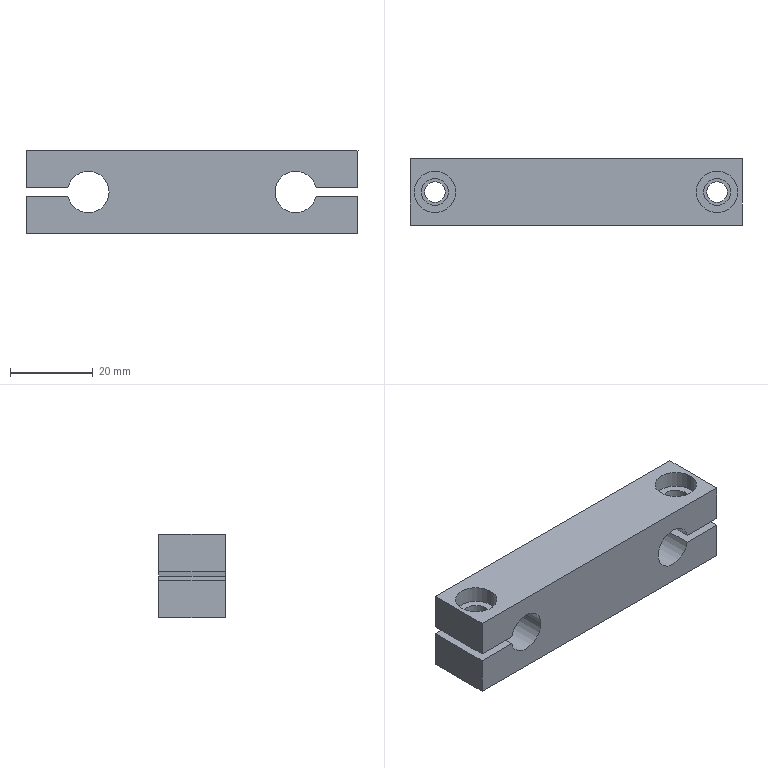Part | SolidWorks | features ICE 4, Extrusion 1, HoleWzd 1 | 1 solid | 29 faces | box 80 x 16 x 20 mm | volume 21131 mm3 | cylinder 15 | plane 14 | commonest cylinder face diameters 10 x7 5 x4 6.5 x4
STEP:
#1=CARTESIAN_POINT('',(-79.,8.,16.));
#2=VERTEX_POINT('',#1);
#3=CARTESIAN_POINT('',(-69.,8.,16.));
#4=VERTEX_POINT('',#3);
#5=CARTESIAN_POINT('',(-74.,8.,16.));
#6=DIRECTION('',(0.,0.,1.));
#7=DIRECTION('',(1.,0.,0.));
#8=AXIS2_PLACEMENT_3D('',#5,#6,#7);
#9=CIRCLE('',#8,5.);
#10=EDGE_CURVE('',#2,#4,#9,.T.);
#11=ORIENTED_EDGE('',*,*,#10,.F.);
#12=CARTESIAN_POINT('',(-79.,8.,20.));
#13=VERTEX_POINT('',#12);
#14=CARTESIAN_POINT('',(-79.,8.,16.));
#15=DIRECTION('',(0.,0.,1.));
#16=VECTOR('',#15,1000.);
#17=LINE('',#14,#16);
#18=EDGE_CURVE('',#2,#13,#17,.T.);
#19=ORIENTED_EDGE('',*,*,#18,.T.);
#20=CARTESIAN_POINT('',(-69.,8.,20.));
#21=VERTEX_POINT('',#20);
#22=CARTESIAN_POINT('',(-74.,8.,20.));
#23=DIRECTION('',(0.,0.,1.));
#24=DIRECTION('',(1.,0.,0.));
#25=AXIS2_PLACEMENT_3D('',#22,#23,#24);
#26=CIRCLE('',#25,5.);
#27=EDGE_CURVE('',#13,#21,#26,.T.);
#28=ORIENTED_EDGE('',*,*,#27,.T.);
#29=CARTESIAN_POINT('',(-69.,8.,16.));
#30=DIRECTION('',(0.,0.,1.));
#31=VECTOR('',#30,1000.);
#32=LINE('',#29,#31);
#33=EDGE_CURVE('',#4,#21,#32,.T.);
#34=ORIENTED_EDGE('',*,*,#33,.F.);
#35=EDGE_LOOP('',(#11,#19,#28,#34));
#36=FACE_OUTER_BOUND('',#35,.T.);
#37=CARTESIAN_POINT('',(-74.,8.,16.));
#38=DIRECTION('',(0.,0.,1.));
#39=DIRECTION('',(1.,0.,0.));
#40=AXIS2_PLACEMENT_3D('',#37,#38,#39);
#41=CYLINDRICAL_SURFACE('',#40,5.);
#42=ADVANCED_FACE('',(#36),#41,.F.);
#43=CARTESIAN_POINT('',(-11.,8.,16.));
#44=VERTEX_POINT('',#43);
#45=CARTESIAN_POINT('',(-1.,8.,16.));
#46=VERTEX_POINT('',#45);
#47=CARTESIAN_POINT('',(-6.,8.,16.));
#48=DIRECTION('',(0.,0.,1.));
#49=DIRECTION('',(1.,0.,0.));
#50=AXIS2_PLACEMENT_3D('',#47,#48,#49);
#51=CIRCLE('',#50,5.);
#52=EDGE_CURVE('',#44,#46,#51,.T.);
#53=ORIENTED_EDGE('',*,*,#52,.F.);
#54=CARTESIAN_POINT('',(-11.,8.,20.));
#55=VERTEX_POINT('',#54);
#56=CARTESIAN_POINT('',(-11.,8.,16.));
#57=DIRECTION('',(0.,0.,1.));
#58=VECTOR('',#57,1000.);
#59=LINE('',#56,#58);
#60=EDGE_CURVE('',#44,#55,#59,.T.);
#61=ORIENTED_EDGE('',*,*,#60,.T.);
#62=CARTESIAN_POINT('',(-1.,8.,20.));
#63=VERTEX_POINT('',#62);
#64=CARTESIAN_POINT('',(-6.,8.,20.));
#65=DIRECTION('',(0.,0.,1.));
#66=DIRECTION('',(1.,0.,0.));
#67=AXIS2_PLACEMENT_3D('',#64,#65,#66);
#68=CIRCLE('',#67,5.);
#69=EDGE_CURVE('',#55,#63,#68,.T.);
#70=ORIENTED_EDGE('',*,*,#69,.T.);
#71=CARTESIAN_POINT('',(-1.,8.,16.));
#72=DIRECTION('',(0.,0.,1.));
#73=VECTOR('',#72,1000.);
#74=LINE('',#71,#73);
#75=EDGE_CURVE('',#46,#63,#74,.T.);
#76=ORIENTED_EDGE('',*,*,#75,.F.);
#77=EDGE_LOOP('',(#53,#61,#70,#76));
#78=FACE_OUTER_BOUND('',#77,.T.);
#79=CARTESIAN_POINT('',(-6.,8.,16.));
#80=DIRECTION('',(0.,0.,1.));
#81=DIRECTION('',(1.,0.,0.));
#82=AXIS2_PLACEMENT_3D('',#79,#80,#81);
#83=CYLINDRICAL_SURFACE('',#82,5.);
#84=ADVANCED_FACE('',(#78),#83,.F.);
#85=CARTESIAN_POINT('',(-8.5,8.,0.));
#86=VERTEX_POINT('',#85);
#87=CARTESIAN_POINT('',(-3.5,8.,0.));
#88=VERTEX_POINT('',#87);
#89=CARTESIAN_POINT('',(-6.,8.,0.));
#90=DIRECTION('',(0.,0.,1.));
#91=DIRECTION('',(1.,0.,0.));
#92=AXIS2_PLACEMENT_3D('',#89,#90,#91);
#93=CIRCLE('',#92,2.5);
#94=EDGE_CURVE('',#86,#88,#93,.T.);
#95=ORIENTED_EDGE('',*,*,#94,.F.);
#96=CARTESIAN_POINT('',(-8.5,8.,9.));
#97=VERTEX_POINT('',#96);
#98=CARTESIAN_POINT('',(-8.5,8.,9.));
#99=DIRECTION('',(0.,0.,1.));
#100=VECTOR('',#99,1000.);
#101=LINE('',#98,#100);
#102=EDGE_CURVE('',#86,#97,#101,.T.);
#103=ORIENTED_EDGE('',*,*,#102,.T.);
#104=CARTESIAN_POINT('',(-3.5,8.,9.));
#105=VERTEX_POINT('',#104);
#106=CARTESIAN_POINT('',(-6.,8.,9.));
#107=DIRECTION('',(0.,0.,1.));
#108=DIRECTION('',(1.,0.,0.));
#109=AXIS2_PLACEMENT_3D('',#106,#107,#108);
#110=CIRCLE('',#109,2.5);
#111=EDGE_CURVE('',#97,#105,#110,.T.);
#112=ORIENTED_EDGE('',*,*,#111,.T.);
#113=CARTESIAN_POINT('',(-3.5,8.,9.));
#114=DIRECTION('',(0.,0.,1.));
#115=VECTOR('',#114,1000.);
#116=LINE('',#113,#115);
#117=EDGE_CURVE('',#88,#105,#116,.T.);
#118=ORIENTED_EDGE('',*,*,#117,.F.);
#119=EDGE_LOOP('',(#95,#103,#112,#118));
#120=FACE_OUTER_BOUND('',#119,.T.);
#121=CARTESIAN_POINT('',(-6.,8.,9.));
#122=DIRECTION('',(0.,0.,1.));
#123=DIRECTION('',(1.,0.,0.));
#124=AXIS2_PLACEMENT_3D('',#121,#122,#123);
#125=CYLINDRICAL_SURFACE('',#124,2.5);
#126=ADVANCED_FACE('',(#120),#125,.F.);
#127=CARTESIAN_POINT('',(-76.5,8.,0.));
#128=VERTEX_POINT('',#127);
#129=CARTESIAN_POINT('',(-71.5,8.,0.));
#130=VERTEX_POINT('',#129);
#131=CARTESIAN_POINT('',(-74.,8.,0.));
#132=DIRECTION('',(0.,0.,1.));
#133=DIRECTION('',(1.,0.,0.));
#134=AXIS2_PLACEMENT_3D('',#131,#132,#133);
#135=CIRCLE('',#134,2.5);
#136=EDGE_CURVE('',#128,#130,#135,.T.);
#137=ORIENTED_EDGE('',*,*,#136,.F.);
#138=CARTESIAN_POINT('',(-76.5,8.,9.));
#139=VERTEX_POINT('',#138);
#140=CARTESIAN_POINT('',(-76.5,8.,9.));
#141=DIRECTION('',(0.,0.,1.));
#142=VECTOR('',#141,1000.);
#143=LINE('',#140,#142);
#144=EDGE_CURVE('',#128,#139,#143,.T.);
#145=ORIENTED_EDGE('',*,*,#144,.T.);
#146=CARTESIAN_POINT('',(-71.5,8.,9.));
#147=VERTEX_POINT('',#146);
#148=CARTESIAN_POINT('',(-74.,8.,9.));
#149=DIRECTION('',(0.,0.,1.));
#150=DIRECTION('',(1.,0.,0.));
#151=AXIS2_PLACEMENT_3D('',#148,#149,#150);
#152=CIRCLE('',#151,2.5);
#153=EDGE_CURVE('',#139,#147,#152,.T.);
#154=ORIENTED_EDGE('',*,*,#153,.T.);
#155=CARTESIAN_POINT('',(-71.5,8.,9.));
#156=DIRECTION('',(0.,0.,1.));
#157=VECTOR('',#156,1000.);
#158=LINE('',#155,#157);
#159=EDGE_CURVE('',#130,#147,#158,.T.);
#160=ORIENTED_EDGE('',*,*,#159,.F.);
#161=EDGE_LOOP('',(#137,#145,#154,#160));
#162=FACE_OUTER_BOUND('',#161,.T.);
#163=CARTESIAN_POINT('',(-74.,8.,9.));
#164=DIRECTION('',(0.,0.,1.));
#165=DIRECTION('',(1.,0.,0.));
#166=AXIS2_PLACEMENT_3D('',#163,#164,#165);
#167=CYLINDRICAL_SURFACE('',#166,2.5);
#168=ADVANCED_FACE('',(#162),#167,.F.);
#169=CARTESIAN_POINT('',(-60.,16.,10.));
#170=VERTEX_POINT('',#169);
#171=CARTESIAN_POINT('',(-69.899,16.,11.));
#172=VERTEX_POINT('',#171);
#173=CARTESIAN_POINT('',(-65.,16.,10.));
#174=DIRECTION('',(0.,-1.,0.));
#175=DIRECTION('',(1.,0.,0.));
#176=AXIS2_PLACEMENT_3D('',#173,#174,#175);
#177=CIRCLE('',#176,5.);
#178=EDGE_CURVE('',#170,#172,#177,.T.);
#179=ORIENTED_EDGE('',*,*,#178,.F.);
#180=CARTESIAN_POINT('',(-60.,0.,10.));
#181=VERTEX_POINT('',#180);
#182=CARTESIAN_POINT('',(-60.,20.,10.));
#183=DIRECTION('',(0.,-1.,0.));
#184=VECTOR('',#183,1000.);
#185=LINE('',#182,#184);
#186=EDGE_CURVE('',#170,#181,#185,.T.);
#187=ORIENTED_EDGE('',*,*,#186,.T.);
#188=CARTESIAN_POINT('',(-69.899,0.,11.));
#189=VERTEX_POINT('',#188);
#190=CARTESIAN_POINT('',(-65.,0.,10.));
#191=DIRECTION('',(0.,-1.,0.));
#192=DIRECTION('',(1.,0.,0.));
#193=AXIS2_PLACEMENT_3D('',#190,#191,#192);
#194=CIRCLE('',#193,5.);
#195=EDGE_CURVE('',#181,#189,#194,.T.);
#196=ORIENTED_EDGE('',*,*,#195,.T.);
#197=CARTESIAN_POINT('',(-69.899,20.,11.));
#198=DIRECTION('',(0.,1.,0.));
#199=VECTOR('',#198,1000.);
#200=LINE('',#197,#199);
#201=EDGE_CURVE('',#189,#172,#200,.T.);
#202=ORIENTED_EDGE('',*,*,#201,.T.);
#203=EDGE_LOOP('',(#179,#187,#196,#202));
#204=FACE_OUTER_BOUND('',#203,.T.);
#205=CARTESIAN_POINT('',(-65.,20.,10.));
#206=DIRECTION('',(0.,-1.,0.));
#207=DIRECTION('',(1.,0.,0.));
#208=AXIS2_PLACEMENT_3D('',#205,#206,#207);
#209=CYLINDRICAL_SURFACE('',#208,5.);
#210=ADVANCED_FACE('',(#204),#209,.F.);
#211=CARTESIAN_POINT('',(-2.75,8.,16.));
#212=VERTEX_POINT('',#211);
#213=CARTESIAN_POINT('',(-9.25,8.,16.));
#214=VERTEX_POINT('',#213);
#215=CARTESIAN_POINT('',(-6.,8.,16.));
#216=DIRECTION('',(0.,0.,-1.));
#217=DIRECTION('',(1.,0.,0.));
#218=AXIS2_PLACEMENT_3D('',#215,#216,#217);
#219=CIRCLE('',#218,3.25);
#220=EDGE_CURVE('',#212,#214,#219,.T.);
#221=ORIENTED_EDGE('',*,*,#220,.F.);
#222=CARTESIAN_POINT('',(-2.75,8.,11.));
#223=VERTEX_POINT('',#222);
#224=CARTESIAN_POINT('',(-2.75,8.,41.));
#225=DIRECTION('',(0.,0.,-1.));
#226=VECTOR('',#225,1000.);
#227=LINE('',#224,#226);
#228=EDGE_CURVE('',#212,#223,#227,.T.);
#229=ORIENTED_EDGE('',*,*,#228,.T.);
#230=CARTESIAN_POINT('',(-9.25,8.,11.));
#231=VERTEX_POINT('',#230);
#232=CARTESIAN_POINT('',(-6.,8.,11.));
#233=DIRECTION('',(0.,0.,-1.));
#234=DIRECTION('',(-1.,0.,0.));
#235=AXIS2_PLACEMENT_3D('',#232,#233,#234);
#236=CIRCLE('',#235,3.25);
#237=EDGE_CURVE('',#223,#231,#236,.T.);
#238=ORIENTED_EDGE('',*,*,#237,.T.);
#239=CARTESIAN_POINT('',(-9.25,8.,41.));
#240=DIRECTION('',(0.,0.,-1.));
#241=VECTOR('',#240,1000.);
#242=LINE('',#239,#241);
#243=EDGE_CURVE('',#214,#231,#242,.T.);
#244=ORIENTED_EDGE('',*,*,#243,.F.);
#245=EDGE_LOOP('',(#221,#229,#238,#244));
#246=FACE_OUTER_BOUND('',#245,.T.);
#247=CARTESIAN_POINT('',(-6.,8.,41.));
#248=DIRECTION('',(0.,0.,-1.));
#249=DIRECTION('',(-1.,0.,0.));
#250=AXIS2_PLACEMENT_3D('',#247,#248,#249);
#251=CYLINDRICAL_SURFACE('',#250,3.25);
#252=ADVANCED_FACE('',(#246),#251,.F.);
#253=CARTESIAN_POINT('',(-70.75,8.,16.));
#254=VERTEX_POINT('',#253);
#255=CARTESIAN_POINT('',(-77.25,8.,16.));
#256=VERTEX_POINT('',#255);
#257=CARTESIAN_POINT('',(-74.,8.,16.));
#258=DIRECTION('',(0.,0.,-1.));
#259=DIRECTION('',(1.,0.,0.));
#260=AXIS2_PLACEMENT_3D('',#257,#258,#259);
#261=CIRCLE('',#260,3.25);
#262=EDGE_CURVE('',#254,#256,#261,.T.);
#263=ORIENTED_EDGE('',*,*,#262,.F.);
#264=CARTESIAN_POINT('',(-70.75,8.,11.));
#265=VERTEX_POINT('',#264);
#266=CARTESIAN_POINT('',(-70.75,8.,41.));
#267=DIRECTION('',(0.,0.,-1.));
#268=VECTOR('',#267,1000.);
#269=LINE('',#266,#268);
#270=EDGE_CURVE('',#254,#265,#269,.T.);
#271=ORIENTED_EDGE('',*,*,#270,.T.);
#272=CARTESIAN_POINT('',(-77.25,8.,11.));
#273=VERTEX_POINT('',#272);
#274=CARTESIAN_POINT('',(-74.,8.,11.));
#275=DIRECTION('',(0.,0.,-1.));
#276=DIRECTION('',(-1.,0.,0.));
#277=AXIS2_PLACEMENT_3D('',#274,#275,#276);
#278=CIRCLE('',#277,3.25);
#279=EDGE_CURVE('',#265,#273,#278,.T.);
#280=ORIENTED_EDGE('',*,*,#279,.T.);
#281=CARTESIAN_POINT('',(-77.25,8.,41.));
#282=DIRECTION('',(0.,0.,-1.));
#283=VECTOR('',#282,1000.);
#284=LINE('',#281,#283);
#285=EDGE_CURVE('',#256,#273,#284,.T.);
#286=ORIENTED_EDGE('',*,*,#285,.F.);
#287=EDGE_LOOP('',(#263,#271,#280,#286));
#288=FACE_OUTER_BOUND('',#287,.T.);
#289=CARTESIAN_POINT('',(-74.,8.,41.));
#290=DIRECTION('',(0.,0.,-1.));
#291=DIRECTION('',(-1.,0.,0.));
#292=AXIS2_PLACEMENT_3D('',#289,#290,#291);
#293=CYLINDRICAL_SURFACE('',#292,3.25);
#294=ADVANCED_FACE('',(#288),#293,.F.);
#295=ORIENTED_EDGE('',*,*,#270,.F.);
#296=CARTESIAN_POINT('',(-74.,8.,16.));
#297=DIRECTION('',(0.,0.,-1.));
#298=DIRECTION('',(1.,0.,0.));
#299=AXIS2_PLACEMENT_3D('',#296,#297,#298);
#300=CIRCLE('',#299,3.25);
#301=EDGE_CURVE('',#256,#254,#300,.T.);
#302=ORIENTED_EDGE('',*,*,#301,.F.);
#303=ORIENTED_EDGE('',*,*,#285,.T.);
#304=CARTESIAN_POINT('',(-74.,8.,11.));
#305=DIRECTION('',(0.,0.,-1.));
#306=DIRECTION('',(-1.,0.,0.));
#307=AXIS2_PLACEMENT_3D('',#304,#305,#306);
#308=CIRCLE('',#307,3.25);
#309=EDGE_CURVE('',#273,#265,#308,.T.);
#310=ORIENTED_EDGE('',*,*,#309,.T.);
#311=EDGE_LOOP('',(#295,#302,#303,#310));
#312=FACE_OUTER_BOUND('',#311,.T.);
#313=CARTESIAN_POINT('',(-74.,8.,41.));
#314=DIRECTION('',(0.,0.,-1.));
#315=DIRECTION('',(-1.,0.,0.));
#316=AXIS2_PLACEMENT_3D('',#313,#314,#315);
#317=CYLINDRICAL_SURFACE('',#316,3.25);
#318=ADVANCED_FACE('',(#312),#317,.F.);
#319=ORIENTED_EDGE('',*,*,#228,.F.);
#320=CARTESIAN_POINT('',(-6.,8.,16.));
#321=DIRECTION('',(0.,0.,-1.));
#322=DIRECTION('',(1.,0.,0.));
#323=AXIS2_PLACEMENT_3D('',#320,#321,#322);
#324=CIRCLE('',#323,3.25);
#325=EDGE_CURVE('',#214,#212,#324,.T.);
#326=ORIENTED_EDGE('',*,*,#325,.F.);
#327=ORIENTED_EDGE('',*,*,#243,.T.);
#328=CARTESIAN_POINT('',(-6.,8.,11.));
#329=DIRECTION('',(0.,0.,-1.));
#330=DIRECTION('',(-1.,0.,0.));
#331=AXIS2_PLACEMENT_3D('',#328,#329,#330);
#332=CIRCLE('',#331,3.25);
#333=EDGE_CURVE('',#231,#223,#332,.T.);
#334=ORIENTED_EDGE('',*,*,#333,.T.);
#335=EDGE_LOOP('',(#319,#326,#327,#334));
#336=FACE_OUTER_BOUND('',#335,.T.);
#337=CARTESIAN_POINT('',(-6.,8.,41.));
#338=DIRECTION('',(0.,0.,-1.));
#339=DIRECTION('',(-1.,0.,0.));
#340=AXIS2_PLACEMENT_3D('',#337,#338,#339);
#341=CYLINDRICAL_SURFACE('',#340,3.25);
#342=ADVANCED_FACE('',(#336),#341,.F.);
#343=CARTESIAN_POINT('',(-80.,16.,20.));
#344=VERTEX_POINT('',#343);
#345=CARTESIAN_POINT('',(-80.,16.,11.));
#346=VERTEX_POINT('',#345);
#347=CARTESIAN_POINT('',(-80.,16.,20.));
#348=DIRECTION('',(0.,0.,-1.));
#349=VECTOR('',#348,1000.);
#350=LINE('',#347,#349);
#351=EDGE_CURVE('',#344,#346,#350,.T.);
#352=ORIENTED_EDGE('',*,*,#351,.T.);
#353=CARTESIAN_POINT('',(-80.,0.,11.));
#354=VERTEX_POINT('',#353);
#355=CARTESIAN_POINT('',(-80.,0.,11.));
#356=DIRECTION('',(0.,-1.,0.));
#357=VECTOR('',#356,1000.);
#358=LINE('',#355,#357);
#359=EDGE_CURVE('',#346,#354,#358,.T.);
#360=ORIENTED_EDGE('',*,*,#359,.T.);
#361=CARTESIAN_POINT('',(-80.,0.,20.));
#362=VERTEX_POINT('',#361);
#363=CARTESIAN_POINT('',(-80.,0.,20.));
#364=DIRECTION('',(0.,0.,-1.));
#365=VECTOR('',#364,1000.);
#366=LINE('',#363,#365);
#367=EDGE_CURVE('',#362,#354,#366,.T.);
#368=ORIENTED_EDGE('',*,*,#367,.F.);
#369=CARTESIAN_POINT('',(-80.,0.,20.));
#370=DIRECTION('',(0.,-1.,0.));
#371=VECTOR('',#370,1000.);
#372=LINE('',#369,#371);
#373=EDGE_CURVE('',#344,#362,#372,.T.);
#374=ORIENTED_EDGE('',*,*,#373,.F.);
#375=EDGE_LOOP('',(#352,#360,#368,#374));
#376=FACE_OUTER_BOUND('',#375,.T.);
#377=CARTESIAN_POINT('',(-80.,0.,20.));
#378=DIRECTION('',(1.,0.,0.));
#379=DIRECTION('',(0.,0.,-1.));
#380=AXIS2_PLACEMENT_3D('',#377,#378,#379);
#381=PLANE('',#380);
#382=ADVANCED_FACE('',(#376),#381,.F.);
#383=CARTESIAN_POINT('',(0.,0.,20.));
#384=VERTEX_POINT('',#383);
#385=CARTESIAN_POINT('',(0.,0.,11.));
#386=VERTEX_POINT('',#385);
#387=CARTESIAN_POINT('',(0.,0.,20.));
#388=DIRECTION('',(0.,0.,-1.));
#389=VECTOR('',#388,1000.);
#390=LINE('',#387,#389);
#391=EDGE_CURVE('',#384,#386,#390,.T.);
#392=ORIENTED_EDGE('',*,*,#391,.T.);
#393=CARTESIAN_POINT('',(0.,16.,11.));
#394=VERTEX_POINT('',#393);
#395=CARTESIAN_POINT('',(0.,0.,11.));
#396=DIRECTION('',(0.,1.,0.));
#397=VECTOR('',#396,1000.);
#398=LINE('',#395,#397);
#399=EDGE_CURVE('',#386,#394,#398,.T.);
#400=ORIENTED_EDGE('',*,*,#399,.T.);
#401=CARTESIAN_POINT('',(0.,16.,20.));
#402=VERTEX_POINT('',#401);
#403=CARTESIAN_POINT('',(0.,16.,20.));
#404=DIRECTION('',(0.,0.,-1.));
#405=VECTOR('',#404,1000.);
#406=LINE('',#403,#405);
#407=EDGE_CURVE('',#402,#394,#406,.T.);
#408=ORIENTED_EDGE('',*,*,#407,.F.);
#409=CARTESIAN_POINT('',(0.,0.,20.));
#410=DIRECTION('',(0.,1.,0.));
#411=VECTOR('',#410,1000.);
#412=LINE('',#409,#411);
#413=EDGE_CURVE('',#384,#402,#412,.T.);
#414=ORIENTED_EDGE('',*,*,#413,.F.);
#415=EDGE_LOOP('',(#392,#400,#408,#414));
#416=FACE_OUTER_BOUND('',#415,.T.);
#417=CARTESIAN_POINT('',(0.,0.,20.));
#418=DIRECTION('',(-1.,0.,0.));
#419=DIRECTION('',(0.,0.,1.));
#420=AXIS2_PLACEMENT_3D('',#417,#418,#419);
#421=PLANE('',#420);
#422=ADVANCED_FACE('',(#416),#421,.F.);
#423=CARTESIAN_POINT('',(0.,16.,9.));
#424=VERTEX_POINT('',#423);
#425=CARTESIAN_POINT('',(0.,16.,0.));
#426=VERTEX_POINT('',#425);
#427=CARTESIAN_POINT('',(0.,16.,20.));
#428=DIRECTION('',(0.,0.,-1.));
#429=VECTOR('',#428,1000.);
#430=LINE('',#427,#429);
#431=EDGE_CURVE('',#424,#426,#430,.T.);
#432=ORIENTED_EDGE('',*,*,#431,.F.);
#433=CARTESIAN_POINT('',(0.,0.,9.));
#434=VERTEX_POINT('',#433);
#435=CARTESIAN_POINT('',(0.,0.,9.));
#436=DIRECTION('',(0.,-1.,0.));
#437=VECTOR('',#436,1000.);
#438=LINE('',#435,#437);
#439=EDGE_CURVE('',#424,#434,#438,.T.);
#440=ORIENTED_EDGE('',*,*,#439,.T.);
#441=CARTESIAN_POINT('',(0.,0.,0.));
#442=VERTEX_POINT('',#441);
#443=CARTESIAN_POINT('',(0.,0.,20.));
#444=DIRECTION('',(0.,0.,-1.));
#445=VECTOR('',#444,1000.);
#446=LINE('',#443,#445);
#447=EDGE_CURVE('',#434,#442,#446,.T.);
#448=ORIENTED_EDGE('',*,*,#447,.T.);
#449=CARTESIAN_POINT('',(0.,0.,0.));
#450=DIRECTION('',(0.,1.,0.));
#451=VECTOR('',#450,1000.);
#452=LINE('',#449,#451);
#453=EDGE_CURVE('',#442,#426,#452,.T.);
#454=ORIENTED_EDGE('',*,*,#453,.T.);
#455=EDGE_LOOP('',(#432,#440,#448,#454));
#456=FACE_OUTER_BOUND('',#455,.T.);
#457=CARTESIAN_POINT('',(0.,0.,20.));
#458=DIRECTION('',(-1.,0.,0.));
#459=DIRECTION('',(0.,0.,1.));
#460=AXIS2_PLACEMENT_3D('',#457,#458,#459);
#461=PLANE('',#460);
#462=ADVANCED_FACE('',(#456),#461,.F.);
#463=CARTESIAN_POINT('',(-69.899,16.,9.));
#464=VERTEX_POINT('',#463);
#465=CARTESIAN_POINT('',(-65.,16.,10.));
#466=DIRECTION('',(0.,-1.,0.));
#467=DIRECTION('',(1.,0.,0.));
#468=AXIS2_PLACEMENT_3D('',#465,#466,#467);
#469=CIRCLE('',#468,5.);
#470=EDGE_CURVE('',#464,#170,#469,.T.);
#471=ORIENTED_EDGE('',*,*,#470,.T.);
#472=ORIENTED_EDGE('',*,*,#178,.T.);
#473=CARTESIAN_POINT('',(0.,16.,11.));
#474=DIRECTION('',(-1.,0.,0.));
#475=VECTOR('',#474,1000.);
#476=LINE('',#473,#475);
#477=EDGE_CURVE('',#172,#346,#476,.T.);
#478=ORIENTED_EDGE('',*,*,#477,.T.);
#479=ORIENTED_EDGE('',*,*,#351,.F.);
#480=CARTESIAN_POINT('',(0.,16.,20.));
#481=DIRECTION('',(-1.,0.,0.));
#482=VECTOR('',#481,1000.);
#483=LINE('',#480,#482);
#484=EDGE_CURVE('',#402,#344,#483,.T.);
#485=ORIENTED_EDGE('',*,*,#484,.F.);
#486=ORIENTED_EDGE('',*,*,#407,.T.);
#487=CARTESIAN_POINT('',(-10.101,16.,11.));
#488=VERTEX_POINT('',#487);
#489=CARTESIAN_POINT('',(0.,16.,11.));
#490=DIRECTION('',(-1.,0.,0.));
#491=VECTOR('',#490,1000.);
#492=LINE('',#489,#491);
#493=EDGE_CURVE('',#394,#488,#492,.T.);
#494=ORIENTED_EDGE('',*,*,#493,.T.);
#495=CARTESIAN_POINT('',(-10.101,16.,9.));
#496=VERTEX_POINT('',#495);
#497=CARTESIAN_POINT('',(-15.,16.,10.));
#498=DIRECTION('',(0.,-1.,0.));
#499=DIRECTION('',(1.,0.,0.));
#500=AXIS2_PLACEMENT_3D('',#497,#498,#499);
#501=CIRCLE('',#500,5.);
#502=EDGE_CURVE('',#488,#496,#501,.T.);
#503=ORIENTED_EDGE('',*,*,#502,.T.);
#504=CARTESIAN_POINT('',(0.,16.,9.));
#505=DIRECTION('',(1.,0.,0.));
#506=VECTOR('',#505,1000.);
#507=LINE('',#504,#506);
#508=EDGE_CURVE('',#496,#424,#507,.T.);
#509=ORIENTED_EDGE('',*,*,#508,.T.);
#510=ORIENTED_EDGE('',*,*,#431,.T.);
#511=CARTESIAN_POINT('',(-80.,16.,0.));
#512=VERTEX_POINT('',#511);
#513=CARTESIAN_POINT('',(0.,16.,0.));
#514=DIRECTION('',(-1.,0.,0.));
#515=VECTOR('',#514,1000.);
#516=LINE('',#513,#515);
#517=EDGE_CURVE('',#426,#512,#516,.T.);
#518=ORIENTED_EDGE('',*,*,#517,.T.);
#519=CARTESIAN_POINT('',(-80.,16.,9.));
#520=VERTEX_POINT('',#519);
#521=CARTESIAN_POINT('',(-80.,16.,20.));
#522=DIRECTION('',(0.,0.,-1.));
#523=VECTOR('',#522,1000.);
#524=LINE('',#521,#523);
#525=EDGE_CURVE('',#520,#512,#524,.T.);
#526=ORIENTED_EDGE('',*,*,#525,.F.);
#527=CARTESIAN_POINT('',(0.,16.,9.));
#528=DIRECTION('',(1.,0.,0.));
#529=VECTOR('',#528,1000.);
#530=LINE('',#527,#529);
#531=EDGE_CURVE('',#520,#464,#530,.T.);
#532=ORIENTED_EDGE('',*,*,#531,.T.);
#533=EDGE_LOOP('',(#471,#472,#478,#479,#485,#486,#494,#503,#509,#510,#518,#526,#532));
#534=FACE_OUTER_BOUND('',#533,.T.);
#535=CARTESIAN_POINT('',(0.,16.,20.));
#536=DIRECTION('',(0.,-1.,0.));
#537=DIRECTION('',(1.,0.,0.));
#538=AXIS2_PLACEMENT_3D('',#535,#536,#537);
#539=PLANE('',#538);
#540=ADVANCED_FACE('',(#534),#539,.F.);
#541=CARTESIAN_POINT('',(-80.,0.,9.));
#542=VERTEX_POINT('',#541);
#543=CARTESIAN_POINT('',(-80.,0.,0.));
#544=VERTEX_POINT('',#543);
#545=CARTESIAN_POINT('',(-80.,0.,20.));
#546=DIRECTION('',(0.,0.,-1.));
#547=VECTOR('',#546,1000.);
#548=LINE('',#545,#547);
#549=EDGE_CURVE('',#542,#544,#548,.T.);
#550=ORIENTED_EDGE('',*,*,#549,.F.);
#551=CARTESIAN_POINT('',(-80.,0.,9.));
#552=DIRECTION('',(0.,1.,0.));
#553=VECTOR('',#552,1000.);
#554=LINE('',#551,#553);
#555=EDGE_CURVE('',#542,#520,#554,.T.);
#556=ORIENTED_EDGE('',*,*,#555,.T.);
#557=ORIENTED_EDGE('',*,*,#525,.T.);
#558=CARTESIAN_POINT('',(-80.,0.,0.));
#559=DIRECTION('',(0.,-1.,0.));
#560=VECTOR('',#559,1000.);
#561=LINE('',#558,#560);
#562=EDGE_CURVE('',#512,#544,#561,.T.);
#563=ORIENTED_EDGE('',*,*,#562,.T.);
#564=EDGE_LOOP('',(#550,#556,#557,#563));
#565=FACE_OUTER_BOUND('',#564,.T.);
#566=CARTESIAN_POINT('',(-80.,0.,20.));
#567=DIRECTION('',(1.,0.,0.));
#568=DIRECTION('',(0.,0.,-1.));
#569=AXIS2_PLACEMENT_3D('',#566,#567,#568);
#570=PLANE('',#569);
#571=ADVANCED_FACE('',(#565),#570,.F.);
#572=ORIENTED_EDGE('',*,*,#367,.T.);
#573=CARTESIAN_POINT('',(-69.055,0.,11.));
#574=DIRECTION('',(-1.,0.,0.));
#575=VECTOR('',#574,1000.);
#576=LINE('',#573,#575);
#577=EDGE_CURVE('',#189,#354,#576,.T.);
#578=ORIENTED_EDGE('',*,*,#577,.F.);
#579=ORIENTED_EDGE('',*,*,#195,.F.);
#580=CARTESIAN_POINT('',(-69.899,0.,9.));
#581=VERTEX_POINT('',#580);
#582=CARTESIAN_POINT('',(-65.,0.,10.));
#583=DIRECTION('',(0.,-1.,0.));
#584=DIRECTION('',(1.,0.,0.));
#585=AXIS2_PLACEMENT_3D('',#582,#583,#584);
#586=CIRCLE('',#585,5.);
#587=EDGE_CURVE('',#581,#181,#586,.T.);
#588=ORIENTED_EDGE('',*,*,#587,.F.);
#589=CARTESIAN_POINT('',(-69.055,0.,9.));
#590=DIRECTION('',(1.,0.,0.));
#591=VECTOR('',#590,1000.);
#592=LINE('',#589,#591);
#593=EDGE_CURVE('',#542,#581,#592,.T.);
#594=ORIENTED_EDGE('',*,*,#593,.F.);
#595=ORIENTED_EDGE('',*,*,#549,.T.);
#596=CARTESIAN_POINT('',(0.,0.,0.));
#597=DIRECTION('',(1.,0.,0.));
#598=VECTOR('',#597,1000.);
#599=LINE('',#596,#598);
#600=EDGE_CURVE('',#544,#442,#599,.T.);
#601=ORIENTED_EDGE('',*,*,#600,.T.);
#602=ORIENTED_EDGE('',*,*,#447,.F.);
#603=CARTESIAN_POINT('',(-10.101,0.,9.));
#604=VERTEX_POINT('',#603);
#605=CARTESIAN_POINT('',(-10.945,0.,9.));
#606=DIRECTION('',(1.,0.,0.));
#607=VECTOR('',#606,1000.);
#608=LINE('',#605,#607);
#609=EDGE_CURVE('',#604,#434,#608,.T.);
#610=ORIENTED_EDGE('',*,*,#609,.F.);
#611=CARTESIAN_POINT('',(-10.101,0.,11.));
#612=VERTEX_POINT('',#611);
#613=CARTESIAN_POINT('',(-15.,0.,10.));
#614=DIRECTION('',(0.,-1.,0.));
#615=DIRECTION('',(1.,0.,0.));
#616=AXIS2_PLACEMENT_3D('',#613,#614,#615);
#617=CIRCLE('',#616,5.);
#618=EDGE_CURVE('',#612,#604,#617,.T.);
#619=ORIENTED_EDGE('',*,*,#618,.F.);
#620=CARTESIAN_POINT('',(-10.945,0.,11.));
#621=DIRECTION('',(-1.,0.,0.));
#622=VECTOR('',#621,1000.);
#623=LINE('',#620,#622);
#624=EDGE_CURVE('',#386,#612,#623,.T.);
#625=ORIENTED_EDGE('',*,*,#624,.F.);
#626=ORIENTED_EDGE('',*,*,#391,.F.);
#627=CARTESIAN_POINT('',(0.,0.,20.));
#628=DIRECTION('',(1.,0.,0.));
#629=VECTOR('',#628,1000.);
#630=LINE('',#627,#629);
#631=EDGE_CURVE('',#362,#384,#630,.T.);
#632=ORIENTED_EDGE('',*,*,#631,.F.);
#633=EDGE_LOOP('',(#572,#578,#579,#588,#594,#595,#601,#602,#610,#619,#625,#626,#632));
#634=FACE_OUTER_BOUND('',#633,.T.);
#635=CARTESIAN_POINT('',(0.,0.,20.));
#636=DIRECTION('',(0.,1.,0.));
#637=DIRECTION('',(-1.,0.,0.));
#638=AXIS2_PLACEMENT_3D('',#635,#636,#637);
#639=PLANE('',#638);
#640=ADVANCED_FACE('',(#634),#639,.F.);
#641=CARTESIAN_POINT('',(-74.,8.,20.));
#642=DIRECTION('',(0.,0.,1.));
#643=DIRECTION('',(1.,0.,0.));
#644=AXIS2_PLACEMENT_3D('',#641,#642,#643);
#645=CIRCLE('',#644,5.);
#646=EDGE_CURVE('',#21,#13,#645,.T.);
#647=ORIENTED_EDGE('',*,*,#646,.F.);
#648=ORIENTED_EDGE('',*,*,#27,.F.);
#649=EDGE_LOOP('',(#647,#648));
#650=FACE_BOUND('',#649,.T.);
#651=CARTESIAN_POINT('',(-6.,8.,20.));
#652=DIRECTION('',(0.,0.,1.));
#653=DIRECTION('',(1.,0.,0.));
#654=AXIS2_PLACEMENT_3D('',#651,#652,#653);
#655=CIRCLE('',#654,5.);
#656=EDGE_CURVE('',#63,#55,#655,.T.);
#657=ORIENTED_EDGE('',*,*,#656,.F.);
#658=ORIENTED_EDGE('',*,*,#69,.F.);
#659=EDGE_LOOP('',(#657,#658));
#660=FACE_BOUND('',#659,.T.);
#661=ORIENTED_EDGE('',*,*,#413,.T.);
#662=ORIENTED_EDGE('',*,*,#484,.T.);
#663=ORIENTED_EDGE('',*,*,#373,.T.);
#664=ORIENTED_EDGE('',*,*,#631,.T.);
#665=EDGE_LOOP('',(#661,#662,#663,#664));
#666=FACE_OUTER_BOUND('',#665,.T.);
#667=CARTESIAN_POINT('',(0.,0.,20.));
#668=DIRECTION('',(0.,0.,1.));
#669=DIRECTION('',(1.,0.,0.));
#670=AXIS2_PLACEMENT_3D('',#667,#668,#669);
#671=PLANE('',#670);
#672=ADVANCED_FACE('',(#650,#660,#666),#671,.T.);
#673=CARTESIAN_POINT('',(-6.,8.,0.));
#674=DIRECTION('',(0.,0.,1.));
#675=DIRECTION('',(1.,0.,0.));
#676=AXIS2_PLACEMENT_3D('',#673,#674,#675);
#677=CIRCLE('',#676,2.5);
#678=EDGE_CURVE('',#88,#86,#677,.T.);
#679=ORIENTED_EDGE('',*,*,#678,.T.);
#680=ORIENTED_EDGE('',*,*,#94,.T.);
#681=EDGE_LOOP('',(#679,#680));
#682=FACE_BOUND('',#681,.T.);
#683=CARTESIAN_POINT('',(-74.,8.,0.));
#684=DIRECTION('',(0.,0.,1.));
#685=DIRECTION('',(1.,0.,0.));
#686=AXIS2_PLACEMENT_3D('',#683,#684,#685);
#687=CIRCLE('',#686,2.5);
#688=EDGE_CURVE('',#130,#128,#687,.T.);
#689=ORIENTED_EDGE('',*,*,#688,.T.);
#690=ORIENTED_EDGE('',*,*,#136,.T.);
#691=EDGE_LOOP('',(#689,#690));
#692=FACE_BOUND('',#691,.T.);
#693=ORIENTED_EDGE('',*,*,#453,.F.);
#694=ORIENTED_EDGE('',*,*,#600,.F.);
#695=ORIENTED_EDGE('',*,*,#562,.F.);
#696=ORIENTED_EDGE('',*,*,#517,.F.);
#697=EDGE_LOOP('',(#693,#694,#695,#696));
#698=FACE_OUTER_BOUND('',#697,.T.);
#699=CARTESIAN_POINT('',(0.,0.,0.));
#700=DIRECTION('',(0.,0.,1.));
#701=DIRECTION('',(1.,0.,0.));
#702=AXIS2_PLACEMENT_3D('',#699,#700,#701);
#703=PLANE('',#702);
#704=ADVANCED_FACE('',(#682,#692,#698),#703,.F.);
#705=ORIENTED_EDGE('',*,*,#502,.F.);
#706=CARTESIAN_POINT('',(-10.101,20.,11.));
#707=DIRECTION('',(0.,-1.,0.));
#708=VECTOR('',#707,1000.);
#709=LINE('',#706,#708);
#710=EDGE_CURVE('',#488,#612,#709,.T.);
#711=ORIENTED_EDGE('',*,*,#710,.T.);
#712=ORIENTED_EDGE('',*,*,#618,.T.);
#713=CARTESIAN_POINT('',(-10.101,20.,9.));
#714=DIRECTION('',(0.,1.,0.));
#715=VECTOR('',#714,1000.);
#716=LINE('',#713,#715);
#717=EDGE_CURVE('',#604,#496,#716,.T.);
#718=ORIENTED_EDGE('',*,*,#717,.T.);
#719=EDGE_LOOP('',(#705,#711,#712,#718));
#720=FACE_OUTER_BOUND('',#719,.T.);
#721=CARTESIAN_POINT('',(-15.,20.,10.));
#722=DIRECTION('',(0.,-1.,0.));
#723=DIRECTION('',(1.,0.,0.));
#724=AXIS2_PLACEMENT_3D('',#721,#722,#723);
#725=CYLINDRICAL_SURFACE('',#724,5.);
#726=ADVANCED_FACE('',(#720),#725,.F.);
#727=ORIENTED_EDGE('',*,*,#186,.F.);
#728=ORIENTED_EDGE('',*,*,#470,.F.);
#729=CARTESIAN_POINT('',(-69.899,20.,9.));
#730=DIRECTION('',(0.,-1.,0.));
#731=VECTOR('',#730,1000.);
#732=LINE('',#729,#731);
#733=EDGE_CURVE('',#464,#581,#732,.T.);
#734=ORIENTED_EDGE('',*,*,#733,.T.);
#735=ORIENTED_EDGE('',*,*,#587,.T.);
#736=EDGE_LOOP('',(#727,#728,#734,#735));
#737=FACE_OUTER_BOUND('',#736,.T.);
#738=CARTESIAN_POINT('',(-65.,20.,10.));
#739=DIRECTION('',(0.,-1.,0.));
#740=DIRECTION('',(1.,0.,0.));
#741=AXIS2_PLACEMENT_3D('',#738,#739,#740);
#742=CYLINDRICAL_SURFACE('',#741,5.);
#743=ADVANCED_FACE('',(#737),#742,.F.);
#744=CARTESIAN_POINT('',(-6.,8.,9.));
#745=DIRECTION('',(0.,0.,1.));
#746=DIRECTION('',(1.,0.,0.));
#747=AXIS2_PLACEMENT_3D('',#744,#745,#746);
#748=CIRCLE('',#747,2.5);
#749=EDGE_CURVE('',#105,#97,#748,.T.);
#750=ORIENTED_EDGE('',*,*,#749,.F.);
#751=ORIENTED_EDGE('',*,*,#111,.F.);
#752=EDGE_LOOP('',(#750,#751));
#753=FACE_BOUND('',#752,.T.);
#754=ORIENTED_EDGE('',*,*,#508,.F.);
#755=ORIENTED_EDGE('',*,*,#717,.F.);
#756=ORIENTED_EDGE('',*,*,#609,.T.);
#757=ORIENTED_EDGE('',*,*,#439,.F.);
#758=EDGE_LOOP('',(#754,#755,#756,#757));
#759=FACE_OUTER_BOUND('',#758,.T.);
#760=CARTESIAN_POINT('',(-10.945,30.,9.));
#761=DIRECTION('',(0.,0.,-1.));
#762=DIRECTION('',(-1.,0.,0.));
#763=AXIS2_PLACEMENT_3D('',#760,#761,#762);
#764=PLANE('',#763);
#765=ADVANCED_FACE('',(#753,#759),#764,.F.);
#766=ORIENTED_EDGE('',*,*,#333,.F.);
#767=ORIENTED_EDGE('',*,*,#237,.F.);
#768=EDGE_LOOP('',(#766,#767));
#769=FACE_BOUND('',#768,.T.);
#770=ORIENTED_EDGE('',*,*,#624,.T.);
#771=ORIENTED_EDGE('',*,*,#710,.F.);
#772=ORIENTED_EDGE('',*,*,#493,.F.);
#773=ORIENTED_EDGE('',*,*,#399,.F.);
#774=EDGE_LOOP('',(#770,#771,#772,#773));
#775=FACE_OUTER_BOUND('',#774,.T.);
#776=CARTESIAN_POINT('',(-10.945,30.,11.));
#777=DIRECTION('',(0.,0.,1.));
#778=DIRECTION('',(1.,0.,0.));
#779=AXIS2_PLACEMENT_3D('',#776,#777,#778);
#780=PLANE('',#779);
#781=ADVANCED_FACE('',(#769,#775),#780,.F.);
#782=CARTESIAN_POINT('',(-74.,8.,9.));
#783=DIRECTION('',(0.,0.,1.));
#784=DIRECTION('',(1.,0.,0.));
#785=AXIS2_PLACEMENT_3D('',#782,#783,#784);
#786=CIRCLE('',#785,2.5);
#787=EDGE_CURVE('',#147,#139,#786,.T.);
#788=ORIENTED_EDGE('',*,*,#787,.F.);
#789=ORIENTED_EDGE('',*,*,#153,.F.);
#790=EDGE_LOOP('',(#788,#789));
#791=FACE_BOUND('',#790,.T.);
#792=ORIENTED_EDGE('',*,*,#593,.T.);
#793=ORIENTED_EDGE('',*,*,#733,.F.);
#794=ORIENTED_EDGE('',*,*,#531,.F.);
#795=ORIENTED_EDGE('',*,*,#555,.F.);
#796=EDGE_LOOP('',(#792,#793,#794,#795));
#797=FACE_OUTER_BOUND('',#796,.T.);
#798=CARTESIAN_POINT('',(-69.055,30.,9.));
#799=DIRECTION('',(0.,0.,-1.));
#800=DIRECTION('',(-1.,0.,0.));
#801=AXIS2_PLACEMENT_3D('',#798,#799,#800);
#802=PLANE('',#801);
#803=ADVANCED_FACE('',(#791,#797),#802,.F.);
#804=ORIENTED_EDGE('',*,*,#309,.F.);
#805=ORIENTED_EDGE('',*,*,#279,.F.);
#806=EDGE_LOOP('',(#804,#805));
#807=FACE_BOUND('',#806,.T.);
#808=ORIENTED_EDGE('',*,*,#477,.F.);
#809=ORIENTED_EDGE('',*,*,#201,.F.);
#810=ORIENTED_EDGE('',*,*,#577,.T.);
#811=ORIENTED_EDGE('',*,*,#359,.F.);
#812=EDGE_LOOP('',(#808,#809,#810,#811));
#813=FACE_OUTER_BOUND('',#812,.T.);
#814=CARTESIAN_POINT('',(-69.055,30.,11.));
#815=DIRECTION('',(0.,0.,1.));
#816=DIRECTION('',(1.,0.,0.));
#817=AXIS2_PLACEMENT_3D('',#814,#815,#816);
#818=PLANE('',#817);
#819=ADVANCED_FACE('',(#807,#813),#818,.F.);
#820=ORIENTED_EDGE('',*,*,#144,.F.);
#821=ORIENTED_EDGE('',*,*,#688,.F.);
#822=ORIENTED_EDGE('',*,*,#159,.T.);
#823=ORIENTED_EDGE('',*,*,#787,.T.);
#824=EDGE_LOOP('',(#820,#821,#822,#823));
#825=FACE_OUTER_BOUND('',#824,.T.);
#826=CARTESIAN_POINT('',(-74.,8.,9.));
#827=DIRECTION('',(0.,0.,1.));
#828=DIRECTION('',(1.,0.,0.));
#829=AXIS2_PLACEMENT_3D('',#826,#827,#828);
#830=CYLINDRICAL_SURFACE('',#829,2.5);
#831=ADVANCED_FACE('',(#825),#830,.F.);
#832=ORIENTED_EDGE('',*,*,#102,.F.);
#833=ORIENTED_EDGE('',*,*,#678,.F.);
#834=ORIENTED_EDGE('',*,*,#117,.T.);
#835=ORIENTED_EDGE('',*,*,#749,.T.);
#836=EDGE_LOOP('',(#832,#833,#834,#835));
#837=FACE_OUTER_BOUND('',#836,.T.);
#838=CARTESIAN_POINT('',(-6.,8.,9.));
#839=DIRECTION('',(0.,0.,1.));
#840=DIRECTION('',(1.,0.,0.));
#841=AXIS2_PLACEMENT_3D('',#838,#839,#840);
#842=CYLINDRICAL_SURFACE('',#841,2.5);
#843=ADVANCED_FACE('',(#837),#842,.F.);
#844=CARTESIAN_POINT('',(-6.,8.,16.));
#845=DIRECTION('',(0.,0.,1.));
#846=DIRECTION('',(1.,0.,0.));
#847=AXIS2_PLACEMENT_3D('',#844,#845,#846);
#848=CIRCLE('',#847,5.);
#849=EDGE_CURVE('',#46,#44,#848,.T.);
#850=ORIENTED_EDGE('',*,*,#849,.T.);
#851=ORIENTED_EDGE('',*,*,#52,.T.);
#852=EDGE_LOOP('',(#850,#851));
#853=FACE_OUTER_BOUND('',#852,.T.);
#854=ORIENTED_EDGE('',*,*,#325,.T.);
#855=ORIENTED_EDGE('',*,*,#220,.T.);
#856=EDGE_LOOP('',(#854,#855));
#857=FACE_BOUND('',#856,.T.);
#858=CARTESIAN_POINT('',(-6.,8.,16.));
#859=DIRECTION('',(0.,0.,1.));
#860=DIRECTION('',(1.,0.,0.));
#861=AXIS2_PLACEMENT_3D('',#858,#859,#860);
#862=PLANE('',#861);
#863=ADVANCED_FACE('',(#853,#857),#862,.T.);
#864=ORIENTED_EDGE('',*,*,#60,.F.);
#865=ORIENTED_EDGE('',*,*,#849,.F.);
#866=ORIENTED_EDGE('',*,*,#75,.T.);
#867=ORIENTED_EDGE('',*,*,#656,.T.);
#868=EDGE_LOOP('',(#864,#865,#866,#867));
#869=FACE_OUTER_BOUND('',#868,.T.);
#870=CARTESIAN_POINT('',(-6.,8.,16.));
#871=DIRECTION('',(0.,0.,1.));
#872=DIRECTION('',(1.,0.,0.));
#873=AXIS2_PLACEMENT_3D('',#870,#871,#872);
#874=CYLINDRICAL_SURFACE('',#873,5.);
#875=ADVANCED_FACE('',(#869),#874,.F.);
#876=CARTESIAN_POINT('',(-74.,8.,16.));
#877=DIRECTION('',(0.,0.,1.));
#878=DIRECTION('',(1.,0.,0.));
#879=AXIS2_PLACEMENT_3D('',#876,#877,#878);
#880=CIRCLE('',#879,5.);
#881=EDGE_CURVE('',#4,#2,#880,.T.);
#882=ORIENTED_EDGE('',*,*,#881,.T.);
#883=ORIENTED_EDGE('',*,*,#10,.T.);
#884=EDGE_LOOP('',(#882,#883));
#885=FACE_OUTER_BOUND('',#884,.T.);
#886=ORIENTED_EDGE('',*,*,#301,.T.);
#887=ORIENTED_EDGE('',*,*,#262,.T.);
#888=EDGE_LOOP('',(#886,#887));
#889=FACE_BOUND('',#888,.T.);
#890=CARTESIAN_POINT('',(-74.,8.,16.));
#891=DIRECTION('',(0.,0.,1.));
#892=DIRECTION('',(1.,0.,0.));
#893=AXIS2_PLACEMENT_3D('',#890,#891,#892);
#894=PLANE('',#893);
#895=ADVANCED_FACE('',(#885,#889),#894,.T.);
#896=ORIENTED_EDGE('',*,*,#18,.F.);
#897=ORIENTED_EDGE('',*,*,#881,.F.);
#898=ORIENTED_EDGE('',*,*,#33,.T.);
#899=ORIENTED_EDGE('',*,*,#646,.T.);
#900=EDGE_LOOP('',(#896,#897,#898,#899));
#901=FACE_OUTER_BOUND('',#900,.T.);
#902=CARTESIAN_POINT('',(-74.,8.,16.));
#903=DIRECTION('',(0.,0.,1.));
#904=DIRECTION('',(1.,0.,0.));
#905=AXIS2_PLACEMENT_3D('',#902,#903,#904);
#906=CYLINDRICAL_SURFACE('',#905,5.);
#907=ADVANCED_FACE('',(#901),#906,.F.);
#908=CLOSED_SHELL('',(#42,#84,#126,#168,#210,#252,#294,#318,#342,#382,#422,#462,#540,#571,#640,#672,#704,#726,#743,#765,#781,#803,#819,#831,#843,#863,#875,#895,#907));
#909=MANIFOLD_SOLID_BREP('',#908);
#910=CARTESIAN_POINT('',(0.,0.,0.));
#911=DIRECTION('',(0.,0.,1.));
#912=DIRECTION('',(1.,0.,0.));
#913=AXIS2_PLACEMENT_3D('',#910,#911,#912);
#914=(LENGTH_UNIT()NAMED_UNIT(*)SI_UNIT(.MILLI.,.METRE.));
#915=UNCERTAINTY_MEASURE_WITH_UNIT(LENGTH_MEASURE(0.00001),#914,'','');
#916=(NAMED_UNIT(*)PLANE_ANGLE_UNIT()SI_UNIT($,.RADIAN.));
#917=(NAMED_UNIT(*)SI_UNIT($,.STERADIAN.)SOLID_ANGLE_UNIT());
#918=(GEOMETRIC_REPRESENTATION_CONTEXT(3)GLOBAL_UNCERTAINTY_ASSIGNED_CONTEXT((#915))GLOBAL_UNIT_ASSIGNED_CONTEXT((#914,#916,#917))REPRESENTATION_CONTEXT('',''));
#919=ADVANCED_BREP_SHAPE_REPRESENTATION('',(#909,#913),#918);